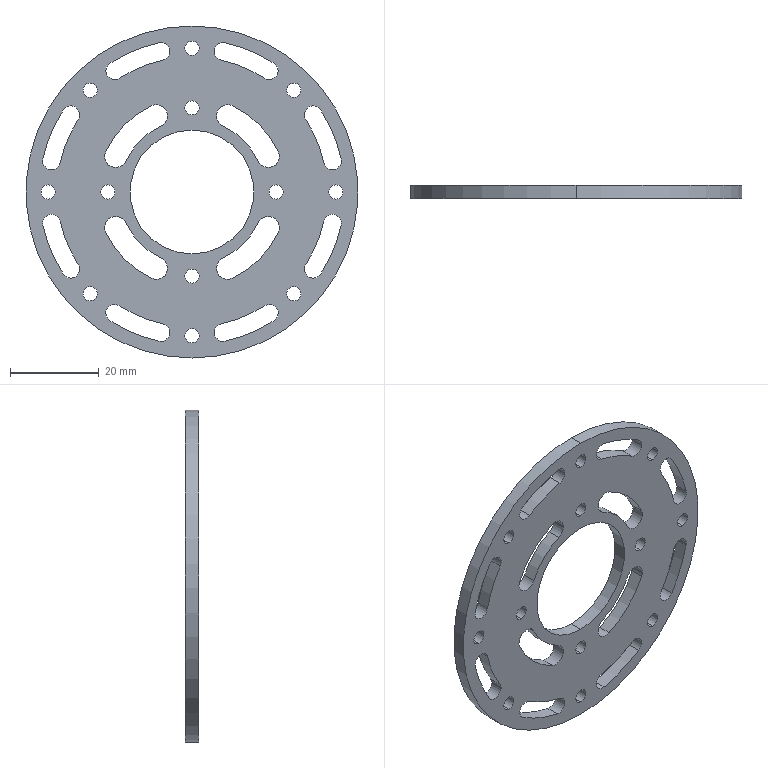Part | SolidWorks | features Extrusion 1, ICE 1 | 1 solid | 90 faces | box 75 x 3 x 75 mm | volume 8695 mm3 | cylinder 88 | plane 2 | commonest cylinder face diameters 3.2 x24 4 x24 5 x12 61 x8 69 x8 33 x4